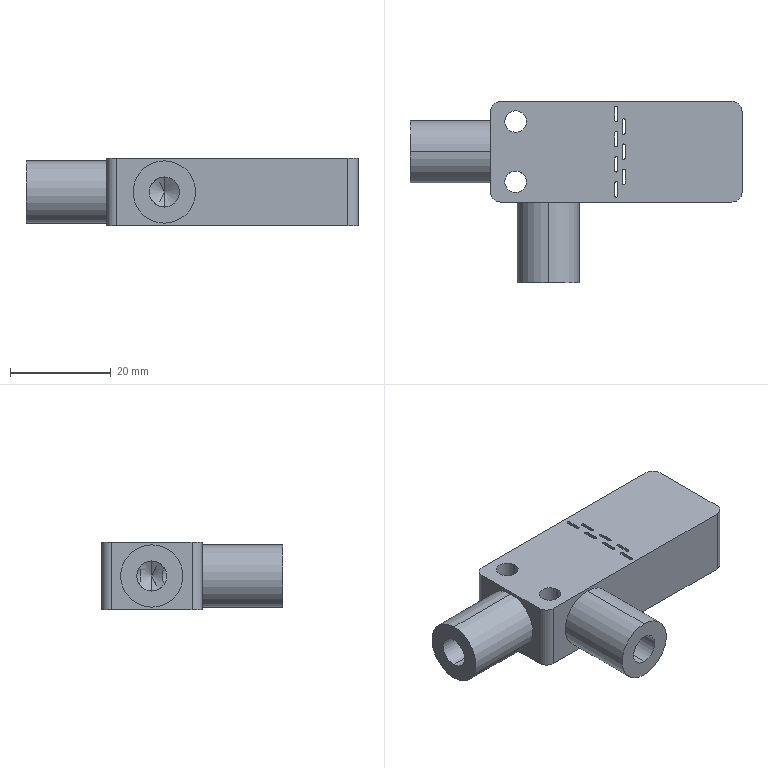Part | SolidWorks | features ICE 4, HoleWzd 3, LPattern 2, Extrusion 1, Fillet 1 | 1 solid | 61 faces | box 66 x 36 x 13.4 mm | volume 15075 mm3 | cylinder 35 | plane 22 | cone 4 | commonest cylinder face diameters 0.6 x14 6 x9 4 x4 4.3 x4 12.4 x4